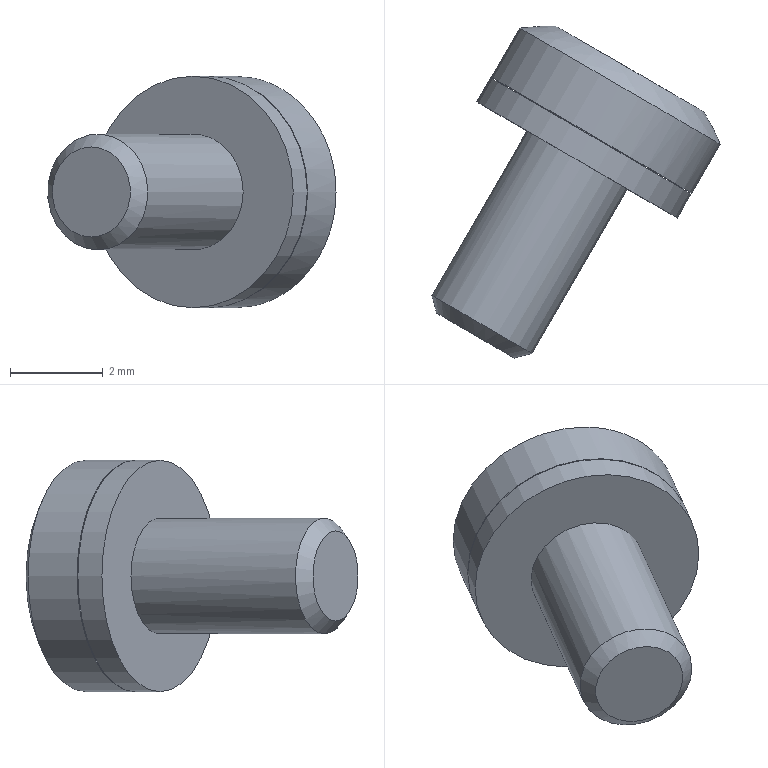Part | STEP file | 1 solid | 24 faces | box 6.225 x 7.171 x 5 mm | volume 60.33 mm3 | cylinder 16 | plane 6 | sphere 1 | cone 1 | commonest cylinder face diameters 0.48 x6 0.84 x6 2.5 x2 5 x2
STEP:
#1=CARTESIAN_POINT('',(8.781,41.105,28.945));
#2=VERTEX_POINT('',#1);
#3=CARTESIAN_POINT('',(9.282,41.97,28.945));
#4=VERTEX_POINT('',#3);
#5=CARTESIAN_POINT('',(8.781,41.105,28.945));
#6=DIRECTION('',(0.5012,0.8653,0.));
#7=VECTOR('',#6,1.);
#8=LINE('',#5,#7);
#9=EDGE_CURVE('',#2,#4,#8,.T.);
#10=ORIENTED_EDGE('',*,*,#9,.T.);
#11=CARTESIAN_POINT('',(9.08,42.087,28.54));
#12=VERTEX_POINT('',#11);
#13=CARTESIAN_POINT('',(9.14,42.053,28.77));
#14=DIRECTION('',(-0.5012,-0.8653,0.));
#15=DIRECTION('',(-0.2481,0.1437,-0.958));
#16=AXIS2_PLACEMENT_3D('',#13,#14,#15);
#17=CIRCLE('',#16,0.24);
#18=EDGE_CURVE('',#12,#4,#17,.T.);
#19=ORIENTED_EDGE('',*,*,#18,.F.);
#20=CARTESIAN_POINT('',(8.579,41.222,28.54));
#21=VERTEX_POINT('',#20);
#22=CARTESIAN_POINT('',(8.579,41.222,28.54));
#23=DIRECTION('',(0.5012,0.8653,0.));
#24=VECTOR('',#23,1.);
#25=LINE('',#22,#24);
#26=EDGE_CURVE('',#21,#12,#25,.T.);
#27=ORIENTED_EDGE('',*,*,#26,.F.);
#28=CARTESIAN_POINT('',(8.639,41.187,28.77));
#29=DIRECTION('',(0.5012,0.8653,0.));
#30=DIRECTION('',(0.5939,-0.344,0.7273));
#31=AXIS2_PLACEMENT_3D('',#28,#29,#30);
#32=CIRCLE('',#31,0.24);
#33=EDGE_CURVE('',#2,#21,#32,.T.);
#34=ORIENTED_EDGE('',*,*,#33,.F.);
#35=EDGE_LOOP('',(#10,#19,#27,#34));
#36=FACE_BOUND('',#35,.T.);
#37=CARTESIAN_POINT('',(9.14,42.053,28.77));
#38=DIRECTION('',(-0.5012,-0.8653,0.));
#39=DIRECTION('',(0.8653,-0.5012,0.));
#40=AXIS2_PLACEMENT_3D('',#37,#38,#39);
#41=CYLINDRICAL_SURFACE('',#40,0.24);
#42=ADVANCED_FACE('',(#36),#41,.F.);
#43=CARTESIAN_POINT('',(8.781,41.105,29.555));
#44=VERTEX_POINT('',#43);
#45=CARTESIAN_POINT('',(9.282,41.97,29.555));
#46=VERTEX_POINT('',#45);
#47=CARTESIAN_POINT('',(8.781,41.105,29.555));
#48=DIRECTION('',(0.5012,0.8653,0.));
#49=VECTOR('',#48,1.);
#50=LINE('',#47,#49);
#51=EDGE_CURVE('',#44,#46,#50,.T.);
#52=ORIENTED_EDGE('',*,*,#51,.T.);
#53=CARTESIAN_POINT('',(9.532,41.826,29.25));
#54=DIRECTION('',(0.5012,0.8653,0.));
#55=DIRECTION('',(-0.5939,0.344,-0.7273));
#56=AXIS2_PLACEMENT_3D('',#53,#54,#55);
#57=CIRCLE('',#56,0.42);
#58=EDGE_CURVE('',#4,#46,#57,.T.);
#59=ORIENTED_EDGE('',*,*,#58,.F.);
#60=ORIENTED_EDGE('',*,*,#9,.F.);
#61=CARTESIAN_POINT('',(9.031,40.96,29.25));
#62=DIRECTION('',(-0.5012,-0.8653,0.));
#63=DIRECTION('',(-0.5939,0.344,0.7273));
#64=AXIS2_PLACEMENT_3D('',#61,#62,#63);
#65=CIRCLE('',#64,0.42);
#66=EDGE_CURVE('',#44,#2,#65,.T.);
#67=ORIENTED_EDGE('',*,*,#66,.F.);
#68=EDGE_LOOP('',(#52,#59,#60,#67));
#69=FACE_BOUND('',#68,.T.);
#70=CARTESIAN_POINT('',(9.532,41.826,29.25));
#71=DIRECTION('',(-0.5012,-0.8653,0.));
#72=DIRECTION('',(0.8653,-0.5012,0.));
#73=AXIS2_PLACEMENT_3D('',#70,#71,#72);
#74=CYLINDRICAL_SURFACE('',#73,0.42);
#75=ADVANCED_FACE('',(#69),#74,.T.);
#76=CARTESIAN_POINT('',(8.579,41.222,29.96));
#77=VERTEX_POINT('',#76);
#78=CARTESIAN_POINT('',(8.639,41.187,29.73));
#79=DIRECTION('',(0.5012,0.8653,0.));
#80=DIRECTION('',(-0.2481,0.1437,0.958));
#81=AXIS2_PLACEMENT_3D('',#78,#79,#80);
#82=CIRCLE('',#81,0.24);
#83=EDGE_CURVE('',#77,#44,#82,.T.);
#84=ORIENTED_EDGE('',*,*,#83,.F.);
#85=CARTESIAN_POINT('',(9.08,42.087,29.96));
#86=VERTEX_POINT('',#85);
#87=CARTESIAN_POINT('',(8.579,41.222,29.96));
#88=DIRECTION('',(0.5012,0.8653,0.));
#89=VECTOR('',#88,1.);
#90=LINE('',#87,#89);
#91=EDGE_CURVE('',#77,#86,#90,.T.);
#92=ORIENTED_EDGE('',*,*,#91,.T.);
#93=CARTESIAN_POINT('',(9.14,42.053,29.73));
#94=DIRECTION('',(-0.5012,-0.8653,0.));
#95=DIRECTION('',(0.5939,-0.344,-0.7273));
#96=AXIS2_PLACEMENT_3D('',#93,#94,#95);
#97=CIRCLE('',#96,0.24);
#98=EDGE_CURVE('',#46,#86,#97,.T.);
#99=ORIENTED_EDGE('',*,*,#98,.F.);
#100=ORIENTED_EDGE('',*,*,#51,.F.);
#101=EDGE_LOOP('',(#84,#92,#99,#100));
#102=FACE_BOUND('',#101,.T.);
#103=CARTESIAN_POINT('',(9.14,42.053,29.73));
#104=DIRECTION('',(-0.5012,-0.8653,0.));
#105=DIRECTION('',(0.8653,-0.5012,0.));
#106=AXIS2_PLACEMENT_3D('',#103,#104,#105);
#107=CYLINDRICAL_SURFACE('',#106,0.24);
#108=ADVANCED_FACE('',(#102),#107,.F.);
#109=CARTESIAN_POINT('',(7.761,42.851,29.96));
#110=VERTEX_POINT('',#109);
#111=CARTESIAN_POINT('',(7.558,42.969,29.555));
#112=VERTEX_POINT('',#111);
#113=CARTESIAN_POINT('',(7.701,42.886,29.73));
#114=DIRECTION('',(-0.5012,-0.8653,0.));
#115=DIRECTION('',(0.2481,-0.1437,0.958));
#116=AXIS2_PLACEMENT_3D('',#113,#114,#115);
#117=CIRCLE('',#116,0.24);
#118=EDGE_CURVE('',#110,#112,#117,.T.);
#119=ORIENTED_EDGE('',*,*,#118,.F.);
#120=CARTESIAN_POINT('',(7.259,41.986,29.96));
#121=VERTEX_POINT('',#120);
#122=CARTESIAN_POINT('',(7.259,41.986,29.96));
#123=DIRECTION('',(0.5012,0.8653,0.));
#124=VECTOR('',#123,1.);
#125=LINE('',#122,#124);
#126=EDGE_CURVE('',#121,#110,#125,.T.);
#127=ORIENTED_EDGE('',*,*,#126,.F.);
#128=CARTESIAN_POINT('',(7.057,42.103,29.555));
#129=VERTEX_POINT('',#128);
#130=CARTESIAN_POINT('',(7.2,42.021,29.73));
#131=DIRECTION('',(0.5012,0.8653,0.));
#132=DIRECTION('',(-0.5939,0.344,-0.7273));
#133=AXIS2_PLACEMENT_3D('',#130,#131,#132);
#134=CIRCLE('',#133,0.24);
#135=EDGE_CURVE('',#129,#121,#134,.T.);
#136=ORIENTED_EDGE('',*,*,#135,.F.);
#137=CARTESIAN_POINT('',(7.057,42.103,29.555));
#138=DIRECTION('',(0.5012,0.8653,0.));
#139=VECTOR('',#138,1.);
#140=LINE('',#137,#139);
#141=EDGE_CURVE('',#129,#112,#140,.T.);
#142=ORIENTED_EDGE('',*,*,#141,.T.);
#143=EDGE_LOOP('',(#119,#127,#136,#142));
#144=FACE_BOUND('',#143,.T.);
#145=CARTESIAN_POINT('',(7.701,42.886,29.73));
#146=DIRECTION('',(-0.5012,-0.8653,0.));
#147=DIRECTION('',(0.8653,-0.5012,0.));
#148=AXIS2_PLACEMENT_3D('',#145,#146,#147);
#149=CYLINDRICAL_SURFACE('',#148,0.24);
#150=ADVANCED_FACE('',(#144),#149,.F.);
#151=ORIENTED_EDGE('',*,*,#141,.F.);
#152=CARTESIAN_POINT('',(7.057,42.103,28.945));
#153=VERTEX_POINT('',#152);
#154=CARTESIAN_POINT('',(6.808,42.248,29.25));
#155=DIRECTION('',(-0.5012,-0.8653,0.));
#156=DIRECTION('',(0.5939,-0.344,-0.7273));
#157=AXIS2_PLACEMENT_3D('',#154,#155,#156);
#158=CIRCLE('',#157,0.42);
#159=EDGE_CURVE('',#153,#129,#158,.T.);
#160=ORIENTED_EDGE('',*,*,#159,.F.);
#161=CARTESIAN_POINT('',(7.558,42.969,28.945));
#162=VERTEX_POINT('',#161);
#163=CARTESIAN_POINT('',(7.057,42.103,28.945));
#164=DIRECTION('',(0.5012,0.8653,0.));
#165=VECTOR('',#164,1.);
#166=LINE('',#163,#165);
#167=EDGE_CURVE('',#153,#162,#166,.T.);
#168=ORIENTED_EDGE('',*,*,#167,.T.);
#169=CARTESIAN_POINT('',(7.309,43.113,29.25));
#170=DIRECTION('',(0.5012,0.8653,0.));
#171=DIRECTION('',(0.5939,-0.344,0.7273));
#172=AXIS2_PLACEMENT_3D('',#169,#170,#171);
#173=CIRCLE('',#172,0.42);
#174=EDGE_CURVE('',#112,#162,#173,.T.);
#175=ORIENTED_EDGE('',*,*,#174,.F.);
#176=EDGE_LOOP('',(#151,#160,#168,#175));
#177=FACE_BOUND('',#176,.T.);
#178=CARTESIAN_POINT('',(7.309,43.113,29.25));
#179=DIRECTION('',(-0.5012,-0.8653,0.));
#180=DIRECTION('',(0.8653,-0.5012,0.));
#181=AXIS2_PLACEMENT_3D('',#178,#179,#180);
#182=CYLINDRICAL_SURFACE('',#181,0.42);
#183=ADVANCED_FACE('',(#177),#182,.T.);
#184=ORIENTED_EDGE('',*,*,#167,.F.);
#185=CARTESIAN_POINT('',(7.259,41.986,28.54));
#186=VERTEX_POINT('',#185);
#187=CARTESIAN_POINT('',(7.2,42.021,28.77));
#188=DIRECTION('',(0.5012,0.8653,0.));
#189=DIRECTION('',(0.2481,-0.1437,-0.958));
#190=AXIS2_PLACEMENT_3D('',#187,#188,#189);
#191=CIRCLE('',#190,0.24);
#192=EDGE_CURVE('',#186,#153,#191,.T.);
#193=ORIENTED_EDGE('',*,*,#192,.F.);
#194=CARTESIAN_POINT('',(7.761,42.851,28.54));
#195=VERTEX_POINT('',#194);
#196=CARTESIAN_POINT('',(7.259,41.986,28.54));
#197=DIRECTION('',(0.5012,0.8653,0.));
#198=VECTOR('',#197,1.);
#199=LINE('',#196,#198);
#200=EDGE_CURVE('',#186,#195,#199,.T.);
#201=ORIENTED_EDGE('',*,*,#200,.T.);
#202=CARTESIAN_POINT('',(7.701,42.886,28.77));
#203=DIRECTION('',(-0.5012,-0.8653,0.));
#204=DIRECTION('',(-0.5939,0.344,0.7273));
#205=AXIS2_PLACEMENT_3D('',#202,#203,#204);
#206=CIRCLE('',#205,0.24);
#207=EDGE_CURVE('',#162,#195,#206,.T.);
#208=ORIENTED_EDGE('',*,*,#207,.F.);
#209=EDGE_LOOP('',(#184,#193,#201,#208));
#210=FACE_BOUND('',#209,.T.);
#211=CARTESIAN_POINT('',(7.701,42.886,28.77));
#212=DIRECTION('',(-0.5012,-0.8653,0.));
#213=DIRECTION('',(0.8653,-0.5012,0.));
#214=AXIS2_PLACEMENT_3D('',#211,#212,#213);
#215=CYLINDRICAL_SURFACE('',#214,0.24);
#216=ADVANCED_FACE('',(#210),#215,.F.);
#217=CARTESIAN_POINT('',(10.369,40.846,29.25));
#218=VERTEX_POINT('',#217);
#219=CARTESIAN_POINT('',(8.206,42.099,29.25));
#220=DIRECTION('',(0.5012,0.8653,0.));
#221=DIRECTION('',(0.8653,-0.5012,0.));
#222=AXIS2_PLACEMENT_3D('',#219,#220,#221);
#223=CIRCLE('',#222,2.5);
#224=EDGE_CURVE('',#218,#218,#223,.T.);
#225=ORIENTED_EDGE('',*,*,#224,.T.);
#226=EDGE_LOOP('',(#225));
#227=FACE_OUTER_BOUND('',#226,.T.);
#228=CARTESIAN_POINT('',(10.015,41.545,29.25));
#229=VERTEX_POINT('',#228);
#230=CARTESIAN_POINT('',(8.42,42.469,29.25));
#231=DIRECTION('',(-0.5012,-0.8653,0.));
#232=DIRECTION('',(0.8653,-0.5012,0.));
#233=AXIS2_PLACEMENT_3D('',#230,#231,#232);
#234=CIRCLE('',#233,1.843);
#235=EDGE_CURVE('',#229,#229,#234,.T.);
#236=ORIENTED_EDGE('',*,*,#235,.T.);
#237=EDGE_LOOP('',(#236));
#238=FACE_BOUND('',#237,.T.);
#239=CARTESIAN_POINT('',(6.641,39.397,29.25));
#240=DIRECTION('',(0.8436,0.537,0.));
#241=DIRECTION('',(0.537,-0.8436,0.));
#242=AXIS2_PLACEMENT_3D('',#239,#240,#241);
#243=SPHERICAL_SURFACE('',#242,4.);
#244=ADVANCED_FACE('',(#227,#238),#243,.T.);
#245=ORIENTED_EDGE('',*,*,#235,.F.);
#246=EDGE_LOOP('',(#245));
#247=FACE_BOUND('',#246,.T.);
#248=ORIENTED_EDGE('',*,*,#18,.T.);
#249=ORIENTED_EDGE('',*,*,#58,.T.);
#250=ORIENTED_EDGE('',*,*,#98,.T.);
#251=CARTESIAN_POINT('',(8.622,42.352,30.265));
#252=VERTEX_POINT('',#251);
#253=CARTESIAN_POINT('',(8.976,42.147,30.362));
#254=DIRECTION('',(0.5012,0.8653,0.));
#255=DIRECTION('',(0.2481,-0.1437,-0.958));
#256=AXIS2_PLACEMENT_3D('',#253,#254,#255);
#257=CIRCLE('',#256,0.42);
#258=EDGE_CURVE('',#86,#252,#257,.T.);
#259=ORIENTED_EDGE('',*,*,#258,.T.);
#260=CARTESIAN_POINT('',(8.218,42.586,30.265));
#261=VERTEX_POINT('',#260);
#262=CARTESIAN_POINT('',(8.42,42.469,30.21));
#263=DIRECTION('',(-0.5012,-0.8653,0.));
#264=DIRECTION('',(0.842,-0.4877,0.2308));
#265=AXIS2_PLACEMENT_3D('',#262,#263,#264);
#266=CIRCLE('',#265,0.24);
#267=EDGE_CURVE('',#252,#261,#266,.T.);
#268=ORIENTED_EDGE('',*,*,#267,.T.);
#269=CARTESIAN_POINT('',(7.865,42.791,30.362));
#270=DIRECTION('',(0.5012,0.8653,0.));
#271=DIRECTION('',(0.842,-0.4877,-0.2308));
#272=AXIS2_PLACEMENT_3D('',#269,#270,#271);
#273=CIRCLE('',#272,0.42);
#274=EDGE_CURVE('',#261,#110,#273,.T.);
#275=ORIENTED_EDGE('',*,*,#274,.T.);
#276=ORIENTED_EDGE('',*,*,#118,.T.);
#277=ORIENTED_EDGE('',*,*,#174,.T.);
#278=ORIENTED_EDGE('',*,*,#207,.T.);
#279=CARTESIAN_POINT('',(8.218,42.586,28.235));
#280=VERTEX_POINT('',#279);
#281=CARTESIAN_POINT('',(7.865,42.791,28.138));
#282=DIRECTION('',(0.5012,0.8653,0.));
#283=DIRECTION('',(-0.2481,0.1437,0.958));
#284=AXIS2_PLACEMENT_3D('',#281,#282,#283);
#285=CIRCLE('',#284,0.42);
#286=EDGE_CURVE('',#195,#280,#285,.T.);
#287=ORIENTED_EDGE('',*,*,#286,.T.);
#288=CARTESIAN_POINT('',(8.622,42.352,28.235));
#289=VERTEX_POINT('',#288);
#290=CARTESIAN_POINT('',(8.42,42.469,28.29));
#291=DIRECTION('',(-0.5012,-0.8653,0.));
#292=DIRECTION('',(-0.842,0.4877,-0.2308));
#293=AXIS2_PLACEMENT_3D('',#290,#291,#292);
#294=CIRCLE('',#293,0.24);
#295=EDGE_CURVE('',#280,#289,#294,.T.);
#296=ORIENTED_EDGE('',*,*,#295,.T.);
#297=CARTESIAN_POINT('',(8.976,42.147,28.138));
#298=DIRECTION('',(0.5012,0.8653,0.));
#299=DIRECTION('',(-0.842,0.4877,0.2308));
#300=AXIS2_PLACEMENT_3D('',#297,#298,#299);
#301=CIRCLE('',#300,0.42);
#302=EDGE_CURVE('',#289,#12,#301,.T.);
#303=ORIENTED_EDGE('',*,*,#302,.T.);
#304=EDGE_LOOP('',(#248,#249,#250,#259,#268,#275,#276,#277,#278,#287,#296,#303));
#305=FACE_BOUND('',#304,.T.);
#306=CARTESIAN_POINT('',(8.42,42.469,29.25));
#307=DIRECTION('',(0.5012,0.8653,0.));
#308=DIRECTION('',(0.,0.,-1.));
#309=AXIS2_PLACEMENT_3D('',#306,#307,#308);
#310=PLANE('',#309);
#311=ADVANCED_FACE('',(#247,#305),#310,.T.);
#312=CARTESIAN_POINT('',(8.121,41.487,28.235));
#313=VERTEX_POINT('',#312);
#314=CARTESIAN_POINT('',(8.475,41.282,28.138));
#315=DIRECTION('',(-0.5012,-0.8653,0.));
#316=DIRECTION('',(0.2481,-0.1437,0.958));
#317=AXIS2_PLACEMENT_3D('',#314,#315,#316);
#318=CIRCLE('',#317,0.42);
#319=EDGE_CURVE('',#21,#313,#318,.T.);
#320=ORIENTED_EDGE('',*,*,#319,.F.);
#321=ORIENTED_EDGE('',*,*,#26,.T.);
#322=ORIENTED_EDGE('',*,*,#302,.F.);
#323=CARTESIAN_POINT('',(8.121,41.487,28.235));
#324=DIRECTION('',(0.5012,0.8653,0.));
#325=VECTOR('',#324,1.);
#326=LINE('',#323,#325);
#327=EDGE_CURVE('',#313,#289,#326,.T.);
#328=ORIENTED_EDGE('',*,*,#327,.F.);
#329=EDGE_LOOP('',(#320,#321,#322,#328));
#330=FACE_BOUND('',#329,.T.);
#331=CARTESIAN_POINT('',(8.976,42.147,28.138));
#332=DIRECTION('',(-0.5012,-0.8653,0.));
#333=DIRECTION('',(0.8653,-0.5012,0.));
#334=AXIS2_PLACEMENT_3D('',#331,#332,#333);
#335=CYLINDRICAL_SURFACE('',#334,0.42);
#336=ADVANCED_FACE('',(#330),#335,.T.);
#337=CARTESIAN_POINT('',(7.717,41.721,28.235));
#338=VERTEX_POINT('',#337);
#339=CARTESIAN_POINT('',(7.919,41.604,28.29));
#340=DIRECTION('',(0.5012,0.8653,0.));
#341=DIRECTION('',(0.842,-0.4877,-0.2308));
#342=AXIS2_PLACEMENT_3D('',#339,#340,#341);
#343=CIRCLE('',#342,0.24);
#344=EDGE_CURVE('',#313,#338,#343,.T.);
#345=ORIENTED_EDGE('',*,*,#344,.F.);
#346=ORIENTED_EDGE('',*,*,#327,.T.);
#347=ORIENTED_EDGE('',*,*,#295,.F.);
#348=CARTESIAN_POINT('',(8.218,42.586,28.235));
#349=DIRECTION('',(-0.5012,-0.8653,0.));
#350=VECTOR('',#349,1.);
#351=LINE('',#348,#350);
#352=EDGE_CURVE('',#280,#338,#351,.T.);
#353=ORIENTED_EDGE('',*,*,#352,.T.);
#354=EDGE_LOOP('',(#345,#346,#347,#353));
#355=FACE_BOUND('',#354,.T.);
#356=CARTESIAN_POINT('',(8.42,42.469,28.29));
#357=DIRECTION('',(-0.5012,-0.8653,0.));
#358=DIRECTION('',(0.8653,-0.5012,0.));
#359=AXIS2_PLACEMENT_3D('',#356,#357,#358);
#360=CYLINDRICAL_SURFACE('',#359,0.24);
#361=ADVANCED_FACE('',(#355),#360,.F.);
#362=CARTESIAN_POINT('',(7.363,41.926,28.138));
#363=DIRECTION('',(-0.5012,-0.8653,0.));
#364=DIRECTION('',(0.842,-0.4877,0.2308));
#365=AXIS2_PLACEMENT_3D('',#362,#363,#364);
#366=CIRCLE('',#365,0.42);
#367=EDGE_CURVE('',#338,#186,#366,.T.);
#368=ORIENTED_EDGE('',*,*,#367,.F.);
#369=ORIENTED_EDGE('',*,*,#352,.F.);
#370=ORIENTED_EDGE('',*,*,#286,.F.);
#371=ORIENTED_EDGE('',*,*,#200,.F.);
#372=EDGE_LOOP('',(#368,#369,#370,#371));
#373=FACE_BOUND('',#372,.T.);
#374=CARTESIAN_POINT('',(7.865,42.791,28.138));
#375=DIRECTION('',(-0.5012,-0.8653,0.));
#376=DIRECTION('',(0.8653,-0.5012,0.));
#377=AXIS2_PLACEMENT_3D('',#374,#375,#376);
#378=CYLINDRICAL_SURFACE('',#377,0.42);
#379=ADVANCED_FACE('',(#373),#378,.T.);
#380=CARTESIAN_POINT('',(7.717,41.721,30.265));
#381=VERTEX_POINT('',#380);
#382=CARTESIAN_POINT('',(7.363,41.926,30.362));
#383=DIRECTION('',(-0.5012,-0.8653,0.));
#384=DIRECTION('',(-0.2481,0.1437,-0.958));
#385=AXIS2_PLACEMENT_3D('',#382,#383,#384);
#386=CIRCLE('',#385,0.42);
#387=EDGE_CURVE('',#121,#381,#386,.T.);
#388=ORIENTED_EDGE('',*,*,#387,.F.);
#389=ORIENTED_EDGE('',*,*,#126,.T.);
#390=ORIENTED_EDGE('',*,*,#274,.F.);
#391=CARTESIAN_POINT('',(7.717,41.721,30.265));
#392=DIRECTION('',(0.5012,0.8653,0.));
#393=VECTOR('',#392,1.);
#394=LINE('',#391,#393);
#395=EDGE_CURVE('',#381,#261,#394,.T.);
#396=ORIENTED_EDGE('',*,*,#395,.F.);
#397=EDGE_LOOP('',(#388,#389,#390,#396));
#398=FACE_BOUND('',#397,.T.);
#399=CARTESIAN_POINT('',(7.865,42.791,30.362));
#400=DIRECTION('',(-0.5012,-0.8653,0.));
#401=DIRECTION('',(0.8653,-0.5012,0.));
#402=AXIS2_PLACEMENT_3D('',#399,#400,#401);
#403=CYLINDRICAL_SURFACE('',#402,0.42);
#404=ADVANCED_FACE('',(#398),#403,.T.);
#405=CARTESIAN_POINT('',(8.121,41.487,30.265));
#406=VERTEX_POINT('',#405);
#407=CARTESIAN_POINT('',(7.919,41.604,30.21));
#408=DIRECTION('',(0.5012,0.8653,0.));
#409=DIRECTION('',(-0.842,0.4877,0.2308));
#410=AXIS2_PLACEMENT_3D('',#407,#408,#409);
#411=CIRCLE('',#410,0.24);
#412=EDGE_CURVE('',#381,#406,#411,.T.);
#413=ORIENTED_EDGE('',*,*,#412,.F.);
#414=ORIENTED_EDGE('',*,*,#395,.T.);
#415=ORIENTED_EDGE('',*,*,#267,.F.);
#416=CARTESIAN_POINT('',(8.121,41.487,30.265));
#417=DIRECTION('',(0.5012,0.8653,0.));
#418=VECTOR('',#417,1.);
#419=LINE('',#416,#418);
#420=EDGE_CURVE('',#406,#252,#419,.T.);
#421=ORIENTED_EDGE('',*,*,#420,.F.);
#422=EDGE_LOOP('',(#413,#414,#415,#421));
#423=FACE_BOUND('',#422,.T.);
#424=CARTESIAN_POINT('',(8.42,42.469,30.21));
#425=DIRECTION('',(-0.5012,-0.8653,0.));
#426=DIRECTION('',(0.8653,-0.5012,0.));
#427=AXIS2_PLACEMENT_3D('',#424,#425,#426);
#428=CYLINDRICAL_SURFACE('',#427,0.24);
#429=ADVANCED_FACE('',(#423),#428,.F.);
#430=CARTESIAN_POINT('',(8.475,41.282,30.362));
#431=DIRECTION('',(-0.5012,-0.8653,0.));
#432=DIRECTION('',(-0.842,0.4877,-0.2308));
#433=AXIS2_PLACEMENT_3D('',#430,#431,#432);
#434=CIRCLE('',#433,0.42);
#435=EDGE_CURVE('',#406,#77,#434,.T.);
#436=ORIENTED_EDGE('',*,*,#435,.F.);
#437=ORIENTED_EDGE('',*,*,#420,.T.);
#438=ORIENTED_EDGE('',*,*,#258,.F.);
#439=ORIENTED_EDGE('',*,*,#91,.F.);
#440=EDGE_LOOP('',(#436,#437,#438,#439));
#441=FACE_BOUND('',#440,.T.);
#442=CARTESIAN_POINT('',(8.976,42.147,30.362));
#443=DIRECTION('',(-0.5012,-0.8653,0.));
#444=DIRECTION('',(0.8653,-0.5012,0.));
#445=AXIS2_PLACEMENT_3D('',#442,#443,#444);
#446=CYLINDRICAL_SURFACE('',#445,0.42);
#447=ADVANCED_FACE('',(#441),#446,.T.);
#448=ORIENTED_EDGE('',*,*,#192,.T.);
#449=ORIENTED_EDGE('',*,*,#159,.T.);
#450=ORIENTED_EDGE('',*,*,#135,.T.);
#451=ORIENTED_EDGE('',*,*,#387,.T.);
#452=ORIENTED_EDGE('',*,*,#412,.T.);
#453=ORIENTED_EDGE('',*,*,#435,.T.);
#454=ORIENTED_EDGE('',*,*,#83,.T.);
#455=ORIENTED_EDGE('',*,*,#66,.T.);
#456=ORIENTED_EDGE('',*,*,#33,.T.);
#457=ORIENTED_EDGE('',*,*,#319,.T.);
#458=ORIENTED_EDGE('',*,*,#344,.T.);
#459=ORIENTED_EDGE('',*,*,#367,.T.);
#460=EDGE_LOOP('',(#448,#449,#450,#451,#452,#453,#454,#455,#456,#457,#458,#459));
#461=FACE_BOUND('',#460,.T.);
#462=CARTESIAN_POINT('',(7.919,41.604,29.25));
#463=DIRECTION('',(0.5012,0.8653,0.));
#464=DIRECTION('',(0.,0.,-1.));
#465=AXIS2_PLACEMENT_3D('',#462,#463,#464);
#466=PLANE('',#465);
#467=ADVANCED_FACE('',(#461),#466,.T.);
#468=ORIENTED_EDGE('',*,*,#224,.F.);
#469=EDGE_LOOP('',(#468));
#470=FACE_OUTER_BOUND('',#469,.T.);
#471=CARTESIAN_POINT('',(9.757,39.788,29.25));
#472=VERTEX_POINT('',#471);
#473=CARTESIAN_POINT('',(7.593,41.041,29.25));
#474=DIRECTION('',(-0.5012,-0.8653,0.));
#475=DIRECTION('',(0.8653,-0.5012,0.));
#476=AXIS2_PLACEMENT_3D('',#473,#474,#475);
#477=CIRCLE('',#476,2.5);
#478=EDGE_CURVE('',#472,#472,#477,.T.);
#479=ORIENTED_EDGE('',*,*,#478,.F.);
#480=EDGE_LOOP('',(#479));
#481=FACE_OUTER_BOUND('',#480,.T.);
#482=CARTESIAN_POINT('',(4.909,36.408,29.25));
#483=DIRECTION('',(-0.5012,-0.8653,0.));
#484=DIRECTION('',(0.8653,-0.5012,0.));
#485=AXIS2_PLACEMENT_3D('',#482,#483,#484);
#486=CYLINDRICAL_SURFACE('',#485,2.5);
#487=ADVANCED_FACE('',(#470,#481),#486,.T.);
#488=ORIENTED_EDGE('',*,*,#478,.T.);
#489=EDGE_LOOP('',(#488));
#490=FACE_BOUND('',#489,.T.);
#491=CARTESIAN_POINT('',(8.675,40.415,29.25));
#492=VERTEX_POINT('',#491);
#493=CARTESIAN_POINT('',(7.593,41.041,29.25));
#494=DIRECTION('',(0.5012,0.8653,0.));
#495=DIRECTION('',(-0.8653,0.5012,0.));
#496=AXIS2_PLACEMENT_3D('',#493,#494,#495);
#497=CIRCLE('',#496,1.25);
#498=EDGE_CURVE('',#492,#492,#497,.T.);
#499=ORIENTED_EDGE('',*,*,#498,.T.);
#500=EDGE_LOOP('',(#499));
#501=FACE_BOUND('',#500,.T.);
#502=CARTESIAN_POINT('',(7.593,41.041,29.25));
#503=DIRECTION('',(0.5012,0.8653,0.));
#504=DIRECTION('',(0.,0.,-1.));
#505=AXIS2_PLACEMENT_3D('',#502,#503,#504);
#506=PLANE('',#505);
#507=ADVANCED_FACE('',(#490,#501),#506,.F.);
#508=ORIENTED_EDGE('',*,*,#498,.F.);
#509=EDGE_LOOP('',(#508));
#510=FACE_OUTER_BOUND('',#509,.T.);
#511=CARTESIAN_POINT('',(8.665,40.398,29.25));
#512=VERTEX_POINT('',#511);
#513=CARTESIAN_POINT('',(7.583,41.024,29.25));
#514=DIRECTION('',(-0.5012,-0.8653,0.));
#515=DIRECTION('',(0.8653,-0.5012,0.));
#516=AXIS2_PLACEMENT_3D('',#513,#514,#515);
#517=CIRCLE('',#516,1.25);
#518=EDGE_CURVE('',#512,#512,#517,.T.);
#519=ORIENTED_EDGE('',*,*,#518,.F.);
#520=EDGE_LOOP('',(#519));
#521=FACE_OUTER_BOUND('',#520,.T.);
#522=CARTESIAN_POINT('',(4.909,36.408,29.25));
#523=DIRECTION('',(-0.5012,-0.8653,0.));
#524=DIRECTION('',(0.8653,-0.5012,0.));
#525=AXIS2_PLACEMENT_3D('',#522,#523,#524);
#526=CYLINDRICAL_SURFACE('',#525,1.25);
#527=ADVANCED_FACE('',(#510,#521),#526,.T.);
#528=CARTESIAN_POINT('',(7.583,41.024,31.75));
#529=VERTEX_POINT('',#528);
#530=CARTESIAN_POINT('',(7.583,41.024,29.25));
#531=DIRECTION('',(0.5012,0.8653,0.));
#532=DIRECTION('',(0.,0.,-1.));
#533=AXIS2_PLACEMENT_3D('',#530,#531,#532);
#534=CIRCLE('',#533,2.5);
#535=EDGE_CURVE('',#529,#529,#534,.T.);
#536=ORIENTED_EDGE('',*,*,#535,.T.);
#537=EDGE_LOOP('',(#536));
#538=FACE_BOUND('',#537,.T.);
#539=ORIENTED_EDGE('',*,*,#518,.T.);
#540=EDGE_LOOP('',(#539));
#541=FACE_BOUND('',#540,.T.);
#542=CARTESIAN_POINT('',(7.583,41.024,29.25));
#543=DIRECTION('',(0.5012,0.8653,0.));
#544=DIRECTION('',(0.,0.,-1.));
#545=AXIS2_PLACEMENT_3D('',#542,#543,#544);
#546=PLANE('',#545);
#547=ADVANCED_FACE('',(#538,#541),#546,.T.);
#548=ORIENTED_EDGE('',*,*,#535,.F.);
#549=EDGE_LOOP('',(#548));
#550=FACE_OUTER_BOUND('',#549,.T.);
#551=CARTESIAN_POINT('',(7.283,40.505,31.75));
#552=VERTEX_POINT('',#551);
#553=CARTESIAN_POINT('',(7.283,40.505,29.25));
#554=DIRECTION('',(-0.5012,-0.8653,0.));
#555=DIRECTION('',(0.,0.,1.));
#556=AXIS2_PLACEMENT_3D('',#553,#554,#555);
#557=CIRCLE('',#556,2.5);
#558=EDGE_CURVE('',#552,#552,#557,.T.);
#559=ORIENTED_EDGE('',*,*,#558,.F.);
#560=EDGE_LOOP('',(#559));
#561=FACE_OUTER_BOUND('',#560,.T.);
#562=CARTESIAN_POINT('',(7.268,40.479,29.25));
#563=DIRECTION('',(-0.5012,-0.8653,0.));
#564=DIRECTION('',(0.,0.,-1.));
#565=AXIS2_PLACEMENT_3D('',#562,#563,#564);
#566=CYLINDRICAL_SURFACE('',#565,2.5);
#567=ADVANCED_FACE('',(#550,#561),#566,.T.);
#568=ORIENTED_EDGE('',*,*,#558,.T.);
#569=EDGE_LOOP('',(#568));
#570=FACE_BOUND('',#569,.T.);
#571=CARTESIAN_POINT('',(8.364,39.878,29.25));
#572=VERTEX_POINT('',#571);
#573=CARTESIAN_POINT('',(7.283,40.505,29.25));
#574=DIRECTION('',(0.5012,0.8653,0.));
#575=DIRECTION('',(-0.8653,0.5012,0.));
#576=AXIS2_PLACEMENT_3D('',#573,#574,#575);
#577=CIRCLE('',#576,1.25);
#578=EDGE_CURVE('',#572,#572,#577,.T.);
#579=ORIENTED_EDGE('',*,*,#578,.T.);
#580=EDGE_LOOP('',(#579));
#581=FACE_BOUND('',#580,.T.);
#582=CARTESIAN_POINT('',(7.283,40.505,29.25));
#583=DIRECTION('',(0.5012,0.8653,0.));
#584=DIRECTION('',(0.,0.,-1.));
#585=AXIS2_PLACEMENT_3D('',#582,#583,#584);
#586=PLANE('',#585);
#587=ADVANCED_FACE('',(#570,#581),#586,.F.);
#588=ORIENTED_EDGE('',*,*,#578,.F.);
#589=EDGE_LOOP('',(#588));
#590=FACE_OUTER_BOUND('',#589,.T.);
#591=CARTESIAN_POINT('',(5.226,36.954,28.));
#592=VERTEX_POINT('',#591);
#593=CARTESIAN_POINT('',(6.307,36.327,29.25));
#594=VERTEX_POINT('',#593);
#595=CARTESIAN_POINT('',(5.226,36.954,29.25));
#596=DIRECTION('',(-0.5012,-0.8653,0.));
#597=DIRECTION('',(0.,0.,-1.));
#598=AXIS2_PLACEMENT_3D('',#595,#596,#597);
#599=CIRCLE('',#598,1.25);
#600=EDGE_CURVE('',#592,#594,#599,.T.);
#601=ORIENTED_EDGE('',*,*,#600,.F.);
#602=CARTESIAN_POINT('',(6.307,36.327,29.25));
#603=CARTESIAN_POINT('',(6.307,36.327,29.276));
#604=CARTESIAN_POINT('',(6.306,36.328,29.329));
#605=CARTESIAN_POINT('',(6.299,36.332,29.407));
#606=CARTESIAN_POINT('',(6.289,36.338,29.484));
#607=CARTESIAN_POINT('',(6.274,36.346,29.561));
#608=CARTESIAN_POINT('',(6.255,36.357,29.637));
#609=CARTESIAN_POINT('',(6.232,36.371,29.711));
#610=CARTESIAN_POINT('',(6.205,36.386,29.783));
#611=CARTESIAN_POINT('',(6.174,36.404,29.853));
#612=CARTESIAN_POINT('',(6.139,36.424,29.92));
#613=CARTESIAN_POINT('',(6.101,36.447,29.985));
#614=CARTESIAN_POINT('',(6.06,36.471,30.047));
#615=CARTESIAN_POINT('',(6.015,36.497,30.106));
#616=CARTESIAN_POINT('',(5.966,36.525,30.162));
#617=CARTESIAN_POINT('',(5.915,36.554,30.214));
#618=CARTESIAN_POINT('',(5.862,36.585,30.262));
#619=CARTESIAN_POINT('',(5.805,36.618,30.306));
#620=CARTESIAN_POINT('',(5.747,36.652,30.346));
#621=CARTESIAN_POINT('',(5.686,36.687,30.382));
#622=CARTESIAN_POINT('',(5.624,36.723,30.413));
#623=CARTESIAN_POINT('',(5.56,36.76,30.44));
#624=CARTESIAN_POINT('',(5.495,36.798,30.462));
#625=CARTESIAN_POINT('',(5.428,36.836,30.479));
#626=CARTESIAN_POINT('',(5.361,36.875,30.491));
#627=CARTESIAN_POINT('',(5.293,36.914,30.498));
#628=CARTESIAN_POINT('',(5.248,36.941,30.5));
#629=CARTESIAN_POINT('',(5.226,36.954,30.5));
#630=CARTESIAN_POINT('',(5.203,36.967,30.5));
#631=CARTESIAN_POINT('',(5.158,36.993,30.498));
#632=CARTESIAN_POINT('',(5.09,37.032,30.491));
#633=CARTESIAN_POINT('',(5.023,37.071,30.479));
#634=CARTESIAN_POINT('',(4.956,37.11,30.462));
#635=CARTESIAN_POINT('',(4.891,37.147,30.44));
#636=CARTESIAN_POINT('',(4.827,37.185,30.413));
#637=CARTESIAN_POINT('',(4.765,37.221,30.382));
#638=CARTESIAN_POINT('',(4.704,37.256,30.346));
#639=CARTESIAN_POINT('',(4.646,37.29,30.306));
#640=CARTESIAN_POINT('',(4.589,37.322,30.262));
#641=CARTESIAN_POINT('',(4.536,37.353,30.214));
#642=CARTESIAN_POINT('',(4.485,37.383,30.162));
#643=CARTESIAN_POINT('',(4.437,37.411,30.106));
#644=CARTESIAN_POINT('',(4.392,37.437,30.047));
#645=CARTESIAN_POINT('',(4.35,37.461,29.985));
#646=CARTESIAN_POINT('',(4.312,37.483,29.92));
#647=CARTESIAN_POINT('',(4.277,37.503,29.852));
#648=CARTESIAN_POINT('',(4.246,37.521,29.782));
#649=CARTESIAN_POINT('',(4.219,37.537,29.71));
#650=CARTESIAN_POINT('',(4.196,37.55,29.636));
#651=CARTESIAN_POINT('',(4.177,37.561,29.561));
#652=CARTESIAN_POINT('',(4.162,37.57,29.484));
#653=CARTESIAN_POINT('',(4.152,37.576,29.406));
#654=CARTESIAN_POINT('',(4.145,37.579,29.328));
#655=CARTESIAN_POINT('',(4.143,37.581,29.25));
#656=CARTESIAN_POINT('',(4.145,37.579,29.171));
#657=CARTESIAN_POINT('',(4.152,37.576,29.093));
#658=CARTESIAN_POINT('',(4.162,37.569,29.015));
#659=CARTESIAN_POINT('',(4.177,37.561,28.939));
#660=CARTESIAN_POINT('',(4.196,37.55,28.863));
#661=CARTESIAN_POINT('',(4.219,37.537,28.789));
#662=CARTESIAN_POINT('',(4.246,37.521,28.717));
#663=CARTESIAN_POINT('',(4.277,37.503,28.647));
#664=CARTESIAN_POINT('',(4.312,37.483,28.579));
#665=CARTESIAN_POINT('',(4.35,37.461,28.514));
#666=CARTESIAN_POINT('',(4.392,37.437,28.452));
#667=CARTESIAN_POINT('',(4.437,37.411,28.393));
#668=CARTESIAN_POINT('',(4.485,37.383,28.338));
#669=CARTESIAN_POINT('',(4.536,37.353,28.286));
#670=CARTESIAN_POINT('',(4.59,37.322,28.238));
#671=CARTESIAN_POINT('',(4.646,37.289,28.194));
#672=CARTESIAN_POINT('',(4.705,37.255,28.154));
#673=CARTESIAN_POINT('',(4.765,37.22,28.118));
#674=CARTESIAN_POINT('',(4.828,37.184,28.087));
#675=CARTESIAN_POINT('',(4.892,37.147,28.06));
#676=CARTESIAN_POINT('',(4.957,37.109,28.038));
#677=CARTESIAN_POINT('',(5.023,37.071,28.021));
#678=CARTESIAN_POINT('',(5.09,37.032,28.009));
#679=CARTESIAN_POINT('',(5.158,36.993,28.002));
#680=CARTESIAN_POINT('',(5.203,36.967,28.));
#681=CARTESIAN_POINT('',(5.226,36.954,28.));
#682=B_SPLINE_CURVE_WITH_KNOTS('',3,(#602,#603,#604,#605,#606,#607,#608,#609,#610,#611,#612,#613,#614,#615,#616,#617,#618,#619,#620,#621,#622,#623,#624,#625,#626,#627,#628,#629,#630,#631,#632,#633,#634,#635,#636,#637,#638,#639,#640,#641,#642,#643,#644,#645,#646,#647,#648,#649,#650,#651,#652,#653,#654,#655,#656,#657,#658,#659,#660,#661,#662,#663,#664,#665,#666,#667,#668,#669,#670,#671,#672,#673,#674,#675,#676,#677,#678,#679,#680,#681),.UNSPECIFIED.,.F.,.F.,(4,1,1,1,1,1,1,1,1,1,1,1,1,1,1,1,1,1,1,1,1,1,1,1,1,3,1,1,1,1,1,1,1,1,1,1,1,1,1,1,1,1,1,1,1,1,1,1,1,1,1,1,1,1,1,1,1,1,1,1,1,1,1,1,1,1,1,1,1,1,1,1,1,1,1,4),(0.,0.01334,0.02667,0.04001,0.05334,0.06668,0.08001,0.09335,0.1067,0.12,0.1334,0.1467,0.16,0.1734,0.1867,0.2,0.2134,0.2267,0.24,0.2534,0.2667,0.28,0.2934,0.3067,0.3201,0.3333,0.3467,0.36,0.3733,0.3867,0.4,0.4133,0.4267,0.44,0.4534,0.4667,0.48,0.4934,0.5067,0.52,0.5334,0.5467,0.56,0.5734,0.5867,0.6,0.6134,0.6267,0.64,0.6534,0.6667,0.6801,0.6934,0.7067,0.7201,0.7334,0.7467,0.7601,0.7734,0.7867,0.8001,0.8134,0.8267,0.8401,0.8534,0.8668,0.8801,0.8934,0.9068,0.9201,0.9334,0.9468,0.9601,0.9734,0.9868,1.),.UNSPECIFIED.);
#683=EDGE_CURVE('',#594,#592,#682,.T.);
#684=ORIENTED_EDGE('',*,*,#683,.F.);
#685=EDGE_LOOP('',(#601,#684));
#686=FACE_BOUND('',#685,.T.);
#687=CARTESIAN_POINT('',(4.909,36.408,29.25));
#688=DIRECTION('',(-0.5012,-0.8653,0.));
#689=DIRECTION('',(0.8653,-0.5012,0.));
#690=AXIS2_PLACEMENT_3D('',#687,#688,#689);
#691=CYLINDRICAL_SURFACE('',#690,1.25);
#692=ADVANCED_FACE('',(#590,#686),#691,.T.);
#693=ORIENTED_EDGE('',*,*,#683,.T.);
#694=ORIENTED_EDGE('',*,*,#600,.T.);
#695=EDGE_LOOP('',(#693,#694));
#696=FACE_BOUND('',#695,.T.);
#697=CARTESIAN_POINT('',(5.087,36.715,28.276));
#698=VERTEX_POINT('',#697);
#699=CARTESIAN_POINT('',(5.087,36.715,29.25));
#700=DIRECTION('',(-0.5012,-0.8653,0.));
#701=DIRECTION('',(0.,0.,-1.));
#702=AXIS2_PLACEMENT_3D('',#699,#700,#701);
#703=CIRCLE('',#702,0.974);
#704=EDGE_CURVE('',#698,#698,#703,.T.);
#705=ORIENTED_EDGE('',*,*,#704,.F.);
#706=EDGE_LOOP('',(#705));
#707=FACE_OUTER_BOUND('',#706,.T.);
#708=CARTESIAN_POINT('',(5.156,36.834,29.25));
#709=DIRECTION('',(0.5012,0.8653,0.));
#710=DIRECTION('',(0.,0.,-1.));
#711=AXIS2_PLACEMENT_3D('',#708,#709,#710);
#712=CONICAL_SURFACE('',#711,1.112,0.7854);
#713=ADVANCED_FACE('',(#696,#707),#712,.T.);
#714=ORIENTED_EDGE('',*,*,#704,.T.);
#715=EDGE_LOOP('',(#714));
#716=FACE_BOUND('',#715,.T.);
#717=CARTESIAN_POINT('',(5.087,36.715,29.25));
#718=DIRECTION('',(0.5012,0.8653,0.));
#719=DIRECTION('',(0.,0.,-1.));
#720=AXIS2_PLACEMENT_3D('',#717,#718,#719);
#721=PLANE('',#720);
#722=ADVANCED_FACE('',(#716),#721,.F.);
#723=CLOSED_SHELL('',(#42,#75,#108,#150,#183,#216,#244,#311,#336,#361,#379,#404,#429,#447,#467,#487,#507,#527,#547,#567,#587,#692,#713,#722));
#724=MANIFOLD_SOLID_BREP('',#723);
#725=(LENGTH_UNIT()NAMED_UNIT(*)SI_UNIT(.MILLI.,.METRE.));
#726=UNCERTAINTY_MEASURE_WITH_UNIT(LENGTH_MEASURE(0.00001),#725,'','');
#727=(NAMED_UNIT(*)PLANE_ANGLE_UNIT()SI_UNIT($,.RADIAN.));
#728=(NAMED_UNIT(*)SI_UNIT($,.STERADIAN.)SOLID_ANGLE_UNIT());
#729=(GEOMETRIC_REPRESENTATION_CONTEXT(3)GLOBAL_UNCERTAINTY_ASSIGNED_CONTEXT((#726))GLOBAL_UNIT_ASSIGNED_CONTEXT((#725,#727,#728))REPRESENTATION_CONTEXT('',''));
#730=ADVANCED_BREP_SHAPE_REPRESENTATION('',(#724),#729);